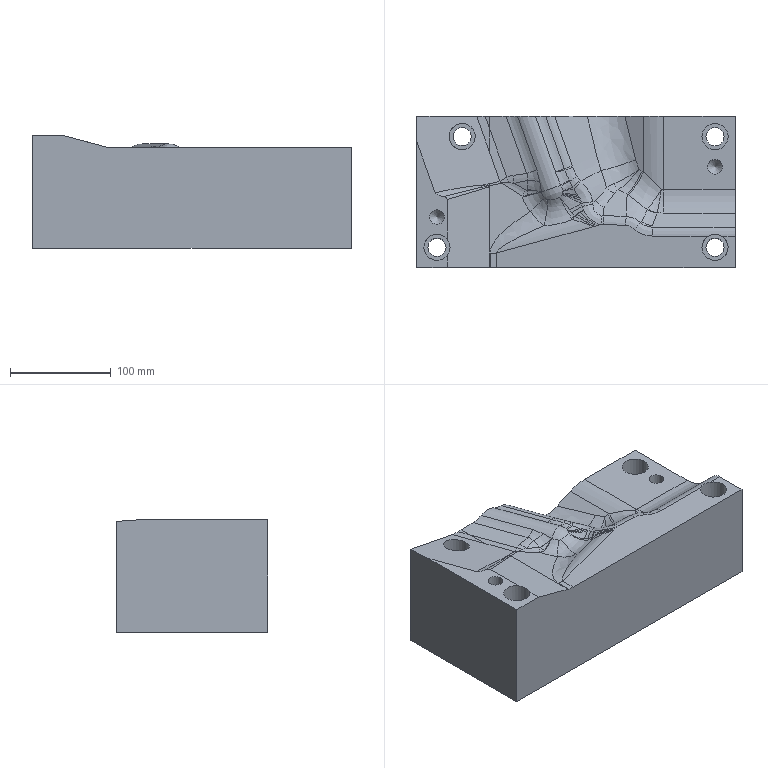Part | STEP file | lll_id5066_x_t | 1 solid | 130 faces | box 316 x 150 x 112 mm | volume 4204871 mm3 | spline 83 | cylinder 24 | plane 19 | cone 2 | sphere 1 | torus 1 | commonest cylinder face diameters 18.009 x4 26.008 x4 25 x3 14.506 x2 45 x2 55 x2